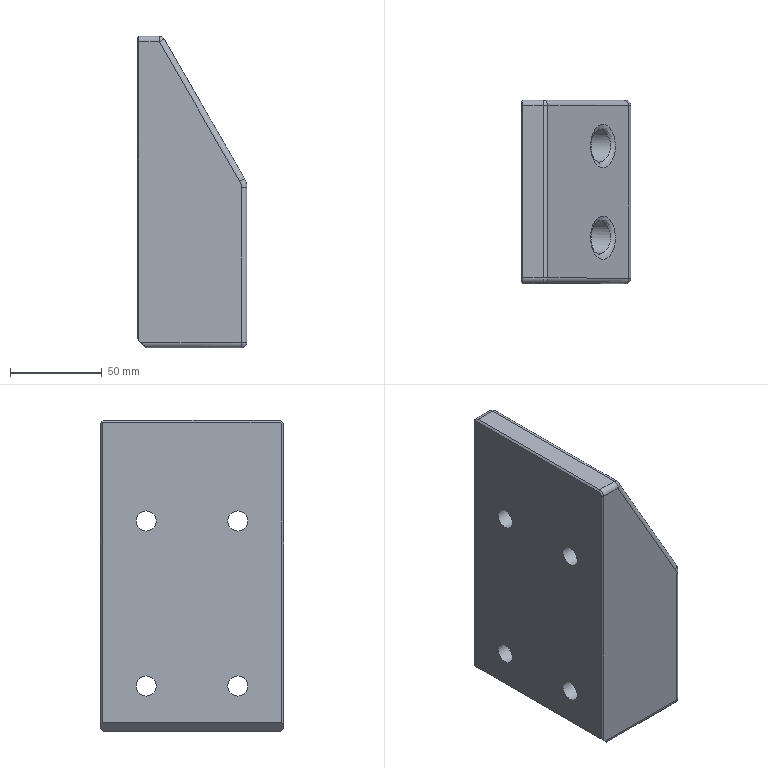Part | NX | features MAIN_BODY 2 | 1 solid | 45 faces | box 60 x 100 x 170 mm | volume 792826 mm3 | cylinder 19 | plane 15 | torus 4 | sphere 4 | spline 2 | cone 1 | commonest cylinder face diameters 6 x10 11 x4 17.5 x4 20 x1
STEP:
#1=CARTESIAN_POINT('',(997.,50.,-147.));
#2=VERTEX_POINT('',#1);
#3=CARTESIAN_POINT('',(996.,50.,-146.));
#4=VERTEX_POINT('',#3);
#5=CARTESIAN_POINT('',(995.,50.,-145.));
#6=DIRECTION('',(0.7071,0.,-0.7071));
#7=VECTOR('',#6,1000.);
#8=LINE('',#5,#7);
#9=EDGE_CURVE('',#2,#4,#8,.F.);
#10=ORIENTED_EDGE('',*,*,#9,.T.);
#11=CARTESIAN_POINT('',(996.,50.,17.));
#12=VERTEX_POINT('',#11);
#13=CARTESIAN_POINT('',(996.,50.,-335.));
#14=DIRECTION('',(0.,0.,1.));
#15=VECTOR('',#14,1000.);
#16=LINE('',#13,#15);
#17=EDGE_CURVE('',#4,#12,#16,.T.);
#18=ORIENTED_EDGE('',*,*,#17,.T.);
#19=CARTESIAN_POINT('',(1007.08,50.,17.));
#20=VERTEX_POINT('',#19);
#21=CARTESIAN_POINT('',(865.,50.,17.));
#22=DIRECTION('',(1.,0.,0.));
#23=VECTOR('',#22,1000.);
#24=LINE('',#21,#23);
#25=EDGE_CURVE('',#12,#20,#24,.T.);
#26=ORIENTED_EDGE('',*,*,#25,.T.);
#27=CARTESIAN_POINT('',(1051.062,50.,-59.179));
#28=VERTEX_POINT('',#27);
#29=CARTESIAN_POINT('',(1051.062,50.,-59.179));
#30=DIRECTION('',(0.5,0.,-0.866));
#31=VECTOR('',#30,1000.);
#32=LINE('',#29,#31);
#33=EDGE_CURVE('',#20,#28,#32,.T.);
#34=ORIENTED_EDGE('',*,*,#33,.T.);
#35=CARTESIAN_POINT('',(1052.,50.,-62.679));
#36=VERTEX_POINT('',#35);
#37=CARTESIAN_POINT('',(1045.,50.,-62.679));
#38=DIRECTION('',(0.,-1.,0.));
#39=DIRECTION('',(1.,0.,0.));
#40=AXIS2_PLACEMENT_3D('',#37,#38,#39);
#41=CIRCLE('',#40,7.);
#42=EDGE_CURVE('',#28,#36,#41,.F.);
#43=ORIENTED_EDGE('',*,*,#42,.T.);
#44=CARTESIAN_POINT('',(1052.,50.,-147.));
#45=VERTEX_POINT('',#44);
#46=CARTESIAN_POINT('',(1052.,50.,-335.));
#47=DIRECTION('',(0.,0.,-1.));
#48=VECTOR('',#47,1000.);
#49=LINE('',#46,#48);
#50=EDGE_CURVE('',#36,#45,#49,.T.);
#51=ORIENTED_EDGE('',*,*,#50,.T.);
#52=CARTESIAN_POINT('',(865.,50.,-147.));
#53=DIRECTION('',(-1.,0.,0.));
#54=VECTOR('',#53,1000.);
#55=LINE('',#52,#54);
#56=EDGE_CURVE('',#45,#2,#55,.T.);
#57=ORIENTED_EDGE('',*,*,#56,.T.);
#58=EDGE_LOOP('',(#10,#18,#26,#34,#43,#51,#57));
#59=FACE_BOUND('',#58,.T.);
#60=CARTESIAN_POINT('',(865.,50.,-335.));
#61=DIRECTION('',(0.,-1.,0.));
#62=DIRECTION('',(0.,0.,1.));
#63=AXIS2_PLACEMENT_3D('',#60,#61,#62);
#64=PLANE('',#63);
#65=ADVANCED_FACE('',(#59),#64,.F.);
#66=CARTESIAN_POINT('',(997.,-50.,-147.));
#67=VERTEX_POINT('',#66);
#68=CARTESIAN_POINT('',(996.,-50.,-146.));
#69=VERTEX_POINT('',#68);
#70=CARTESIAN_POINT('',(995.,-50.,-145.));
#71=DIRECTION('',(-0.7071,0.,0.7071));
#72=VECTOR('',#71,1000.);
#73=LINE('',#70,#72);
#74=EDGE_CURVE('',#67,#69,#73,.T.);
#75=ORIENTED_EDGE('',*,*,#74,.F.);
#76=CARTESIAN_POINT('',(1052.,-50.,-147.));
#77=VERTEX_POINT('',#76);
#78=CARTESIAN_POINT('',(865.,-50.,-147.));
#79=DIRECTION('',(-1.,0.,0.));
#80=VECTOR('',#79,1000.);
#81=LINE('',#78,#80);
#82=EDGE_CURVE('',#77,#67,#81,.T.);
#83=ORIENTED_EDGE('',*,*,#82,.F.);
#84=CARTESIAN_POINT('',(1052.,-50.,-62.679));
#85=VERTEX_POINT('',#84);
#86=CARTESIAN_POINT('',(1052.,-50.,-335.));
#87=DIRECTION('',(0.,0.,1.));
#88=VECTOR('',#87,1000.);
#89=LINE('',#86,#88);
#90=EDGE_CURVE('',#85,#77,#89,.F.);
#91=ORIENTED_EDGE('',*,*,#90,.F.);
#92=CARTESIAN_POINT('',(1051.062,-50.,-59.179));
#93=VERTEX_POINT('',#92);
#94=CARTESIAN_POINT('',(1045.,-50.,-62.679));
#95=DIRECTION('',(0.,1.,0.));
#96=DIRECTION('',(-1.,0.,0.));
#97=AXIS2_PLACEMENT_3D('',#94,#95,#96);
#98=CIRCLE('',#97,7.);
#99=EDGE_CURVE('',#93,#85,#98,.T.);
#100=ORIENTED_EDGE('',*,*,#99,.F.);
#101=CARTESIAN_POINT('',(1007.08,-50.,17.));
#102=VERTEX_POINT('',#101);
#103=CARTESIAN_POINT('',(1051.062,-50.,-59.179));
#104=DIRECTION('',(-0.5,0.,0.866));
#105=VECTOR('',#104,1000.);
#106=LINE('',#103,#105);
#107=EDGE_CURVE('',#102,#93,#106,.F.);
#108=ORIENTED_EDGE('',*,*,#107,.F.);
#109=CARTESIAN_POINT('',(996.,-50.,17.));
#110=VERTEX_POINT('',#109);
#111=CARTESIAN_POINT('',(865.,-50.,17.));
#112=DIRECTION('',(1.,0.,0.));
#113=VECTOR('',#112,1000.);
#114=LINE('',#111,#113);
#115=EDGE_CURVE('',#110,#102,#114,.T.);
#116=ORIENTED_EDGE('',*,*,#115,.F.);
#117=CARTESIAN_POINT('',(996.,-50.,-335.));
#118=DIRECTION('',(0.,0.,-1.));
#119=VECTOR('',#118,1000.);
#120=LINE('',#117,#119);
#121=EDGE_CURVE('',#69,#110,#120,.F.);
#122=ORIENTED_EDGE('',*,*,#121,.F.);
#123=EDGE_LOOP('',(#75,#83,#91,#100,#108,#116,#122));
#124=FACE_BOUND('',#123,.T.);
#125=CARTESIAN_POINT('',(865.,-50.,-335.));
#126=DIRECTION('',(0.,-1.,0.));
#127=DIRECTION('',(0.,0.,1.));
#128=AXIS2_PLACEMENT_3D('',#125,#126,#127);
#129=PLANE('',#128);
#130=ADVANCED_FACE('',(#124),#129,.T.);
#131=CARTESIAN_POINT('',(1055.,25.,-136.75));
#132=VERTEX_POINT('',#131);
#133=CARTESIAN_POINT('',(1055.,25.,-125.));
#134=DIRECTION('',(1.,0.,0.));
#135=DIRECTION('',(0.,0.,-1.));
#136=AXIS2_PLACEMENT_3D('',#133,#134,#135);
#137=CIRCLE('',#136,11.75);
#138=EDGE_CURVE('',#132,#132,#137,.T.);
#139=ORIENTED_EDGE('',*,*,#138,.F.);
#140=EDGE_LOOP('',(#139));
#141=FACE_BOUND('',#140,.T.);
#142=CARTESIAN_POINT('',(1055.,-25.,-136.75));
#143=VERTEX_POINT('',#142);
#144=CARTESIAN_POINT('',(1055.,-25.,-125.));
#145=DIRECTION('',(1.,0.,0.));
#146=DIRECTION('',(0.,0.,-1.));
#147=AXIS2_PLACEMENT_3D('',#144,#145,#146);
#148=CIRCLE('',#147,11.75);
#149=EDGE_CURVE('',#143,#143,#148,.T.);
#150=ORIENTED_EDGE('',*,*,#149,.F.);
#151=EDGE_LOOP('',(#150));
#152=FACE_BOUND('',#151,.T.);
#153=CARTESIAN_POINT('',(1055.,47.,-147.));
#154=VERTEX_POINT('',#153);
#155=CARTESIAN_POINT('',(1055.,-47.,-147.));
#156=VERTEX_POINT('',#155);
#157=CARTESIAN_POINT('',(1055.,0.,-147.));
#158=DIRECTION('',(0.,-1.,0.));
#159=VECTOR('',#158,1000.);
#160=LINE('',#157,#159);
#161=EDGE_CURVE('',#154,#156,#160,.T.);
#162=ORIENTED_EDGE('',*,*,#161,.F.);
#163=CARTESIAN_POINT('',(1055.,47.,-62.679));
#164=VERTEX_POINT('',#163);
#165=CARTESIAN_POINT('',(1055.,47.,-105.));
#166=DIRECTION('',(0.,0.,-1.));
#167=VECTOR('',#166,1000.);
#168=LINE('',#165,#167);
#169=EDGE_CURVE('',#154,#164,#168,.F.);
#170=ORIENTED_EDGE('',*,*,#169,.T.);
#171=CARTESIAN_POINT('',(1055.,-47.,-62.679));
#172=VERTEX_POINT('',#171);
#173=CARTESIAN_POINT('',(1055.,-40.,-62.679));
#174=DIRECTION('',(0.,1.,0.));
#175=VECTOR('',#174,1000.);
#176=LINE('',#173,#175);
#177=EDGE_CURVE('',#164,#172,#176,.F.);
#178=ORIENTED_EDGE('',*,*,#177,.T.);
#179=CARTESIAN_POINT('',(1055.,-47.,-105.));
#180=DIRECTION('',(0.,0.,-1.));
#181=VECTOR('',#180,1000.);
#182=LINE('',#179,#181);
#183=EDGE_CURVE('',#156,#172,#182,.F.);
#184=ORIENTED_EDGE('',*,*,#183,.F.);
#185=EDGE_LOOP('',(#162,#170,#178,#184));
#186=FACE_BOUND('',#185,.T.);
#187=CARTESIAN_POINT('',(1055.,0.,-105.));
#188=DIRECTION('',(-1.,0.,0.));
#189=DIRECTION('',(0.,1.,0.));
#190=AXIS2_PLACEMENT_3D('',#187,#188,#189);
#191=PLANE('',#190);
#192=ADVANCED_FACE('',(#141,#152,#186),#191,.F.);
#193=CARTESIAN_POINT('',(1043.886,25.,-43.75));
#194=VERTEX_POINT('',#193);
#195=CARTESIAN_POINT('',(1037.102,25.,-35.));
#196=DIRECTION('',(0.7903,0.,0.6127));
#197=DIRECTION('',(0.6127,0.,-0.7903));
#198=AXIS2_PLACEMENT_3D('',#195,#196,#197);
#199=ELLIPSE('',#198,11.072,8.75);
#200=EDGE_CURVE('',#194,#194,#199,.F.);
#201=ORIENTED_EDGE('',*,*,#200,.F.);
#202=EDGE_LOOP('',(#201));
#203=FACE_BOUND('',#202,.T.);
#204=CARTESIAN_POINT('',(1015.,25.,-26.25));
#205=VERTEX_POINT('',#204);
#206=CARTESIAN_POINT('',(1015.,25.,-35.));
#207=DIRECTION('',(1.,0.,0.));
#208=DIRECTION('',(0.,0.,1.));
#209=AXIS2_PLACEMENT_3D('',#206,#207,#208);
#210=CIRCLE('',#209,8.75);
#211=EDGE_CURVE('',#205,#205,#210,.T.);
#212=ORIENTED_EDGE('',*,*,#211,.F.);
#213=EDGE_LOOP('',(#212));
#214=FACE_BOUND('',#213,.T.);
#215=CARTESIAN_POINT('',(1020.,25.,-35.));
#216=DIRECTION('',(1.,0.,0.));
#217=DIRECTION('',(0.,0.,1.));
#218=AXIS2_PLACEMENT_3D('',#215,#216,#217);
#219=CYLINDRICAL_SURFACE('',#218,8.75);
#220=ADVANCED_FACE('',(#203,#214),#219,.F.);
#221=CARTESIAN_POINT('',(1043.886,-25.,-43.75));
#222=VERTEX_POINT('',#221);
#223=CARTESIAN_POINT('',(1037.102,-25.,-35.));
#224=DIRECTION('',(0.7903,0.,0.6127));
#225=DIRECTION('',(0.6127,0.,-0.7903));
#226=AXIS2_PLACEMENT_3D('',#223,#224,#225);
#227=ELLIPSE('',#226,11.072,8.75);
#228=EDGE_CURVE('',#222,#222,#227,.F.);
#229=ORIENTED_EDGE('',*,*,#228,.F.);
#230=EDGE_LOOP('',(#229));
#231=FACE_BOUND('',#230,.T.);
#232=CARTESIAN_POINT('',(1015.,-25.,-26.25));
#233=VERTEX_POINT('',#232);
#234=CARTESIAN_POINT('',(1015.,-25.,-35.));
#235=DIRECTION('',(1.,0.,0.));
#236=DIRECTION('',(0.,0.,1.));
#237=AXIS2_PLACEMENT_3D('',#234,#235,#236);
#238=CIRCLE('',#237,8.75);
#239=EDGE_CURVE('',#233,#233,#238,.T.);
#240=ORIENTED_EDGE('',*,*,#239,.F.);
#241=EDGE_LOOP('',(#240));
#242=FACE_BOUND('',#241,.T.);
#243=CARTESIAN_POINT('',(1020.,-25.,-35.));
#244=DIRECTION('',(1.,0.,0.));
#245=DIRECTION('',(0.,0.,1.));
#246=AXIS2_PLACEMENT_3D('',#243,#244,#245);
#247=CYLINDRICAL_SURFACE('',#246,8.75);
#248=ADVANCED_FACE('',(#231,#242),#247,.F.);
#249=CARTESIAN_POINT('',(995.,25.,-29.5));
#250=VERTEX_POINT('',#249);
#251=CARTESIAN_POINT('',(995.,25.,-35.));
#252=DIRECTION('',(1.,0.,0.));
#253=DIRECTION('',(0.,0.,1.));
#254=AXIS2_PLACEMENT_3D('',#251,#252,#253);
#255=CIRCLE('',#254,5.5);
#256=EDGE_CURVE('',#250,#250,#255,.F.);
#257=ORIENTED_EDGE('',*,*,#256,.F.);
#258=EDGE_LOOP('',(#257));
#259=FACE_BOUND('',#258,.T.);
#260=CARTESIAN_POINT('',(995.,25.,-119.5));
#261=VERTEX_POINT('',#260);
#262=CARTESIAN_POINT('',(995.,25.,-125.));
#263=DIRECTION('',(1.,0.,0.));
#264=DIRECTION('',(0.,0.,1.));
#265=AXIS2_PLACEMENT_3D('',#262,#263,#264);
#266=CIRCLE('',#265,5.5);
#267=EDGE_CURVE('',#261,#261,#266,.F.);
#268=ORIENTED_EDGE('',*,*,#267,.F.);
#269=EDGE_LOOP('',(#268));
#270=FACE_BOUND('',#269,.T.);
#271=CARTESIAN_POINT('',(995.,-25.,-119.5));
#272=VERTEX_POINT('',#271);
#273=CARTESIAN_POINT('',(995.,-25.,-125.));
#274=DIRECTION('',(1.,0.,0.));
#275=DIRECTION('',(0.,0.,1.));
#276=AXIS2_PLACEMENT_3D('',#273,#274,#275);
#277=CIRCLE('',#276,5.5);
#278=EDGE_CURVE('',#272,#272,#277,.F.);
#279=ORIENTED_EDGE('',*,*,#278,.F.);
#280=EDGE_LOOP('',(#279));
#281=FACE_BOUND('',#280,.T.);
#282=CARTESIAN_POINT('',(995.,49.,19.));
#283=VERTEX_POINT('',#282);
#284=CARTESIAN_POINT('',(995.,-47.,19.));
#285=VERTEX_POINT('',#284);
#286=CARTESIAN_POINT('',(995.,95.,19.));
#287=DIRECTION('',(0.,-1.,0.));
#288=VECTOR('',#287,1000.);
#289=LINE('',#286,#288);
#290=EDGE_CURVE('',#283,#285,#289,.T.);
#291=ORIENTED_EDGE('',*,*,#290,.F.);
#292=CARTESIAN_POINT('',(995.,49.,-145.));
#293=VERTEX_POINT('',#292);
#294=CARTESIAN_POINT('',(995.,49.,-335.));
#295=DIRECTION('',(0.,0.,-1.));
#296=VECTOR('',#295,1000.);
#297=LINE('',#294,#296);
#298=EDGE_CURVE('',#283,#293,#297,.T.);
#299=ORIENTED_EDGE('',*,*,#298,.T.);
#300=CARTESIAN_POINT('',(995.,-49.,-145.));
#301=VERTEX_POINT('',#300);
#302=CARTESIAN_POINT('',(995.,95.,-145.));
#303=DIRECTION('',(0.,1.,0.));
#304=VECTOR('',#303,1000.);
#305=LINE('',#302,#304);
#306=EDGE_CURVE('',#301,#293,#305,.T.);
#307=ORIENTED_EDGE('',*,*,#306,.F.);
#308=CARTESIAN_POINT('',(995.,-49.,17.));
#309=VERTEX_POINT('',#308);
#310=CARTESIAN_POINT('',(995.,-49.,-335.));
#311=DIRECTION('',(0.,0.,-1.));
#312=VECTOR('',#311,1000.);
#313=LINE('',#310,#312);
#314=EDGE_CURVE('',#309,#301,#313,.T.);
#315=ORIENTED_EDGE('',*,*,#314,.F.);
#316=CARTESIAN_POINT('',(995.,-47.,17.));
#317=DIRECTION('',(-1.,0.,0.));
#318=DIRECTION('',(0.,0.,1.));
#319=AXIS2_PLACEMENT_3D('',#316,#317,#318);
#320=CIRCLE('',#319,2.);
#321=EDGE_CURVE('',#285,#309,#320,.F.);
#322=ORIENTED_EDGE('',*,*,#321,.F.);
#323=EDGE_LOOP('',(#291,#299,#307,#315,#322));
#324=FACE_BOUND('',#323,.T.);
#325=CARTESIAN_POINT('',(995.,-25.,-29.5));
#326=VERTEX_POINT('',#325);
#327=CARTESIAN_POINT('',(995.,-25.,-35.));
#328=DIRECTION('',(1.,0.,0.));
#329=DIRECTION('',(0.,0.,1.));
#330=AXIS2_PLACEMENT_3D('',#327,#328,#329);
#331=CIRCLE('',#330,5.5);
#332=EDGE_CURVE('',#326,#326,#331,.F.);
#333=ORIENTED_EDGE('',*,*,#332,.F.);
#334=EDGE_LOOP('',(#333));
#335=FACE_BOUND('',#334,.T.);
#336=CARTESIAN_POINT('',(995.,95.,-335.));
#337=DIRECTION('',(1.,0.,0.));
#338=DIRECTION('',(0.,-1.,0.));
#339=AXIS2_PLACEMENT_3D('',#336,#337,#338);
#340=PLANE('',#339);
#341=ADVANCED_FACE('',(#259,#270,#281,#324,#335),#340,.F.);
#342=CARTESIAN_POINT('',(1007.08,47.,20.));
#343=VERTEX_POINT('',#342);
#344=CARTESIAN_POINT('',(1007.08,-47.,20.));
#345=VERTEX_POINT('',#344);
#346=CARTESIAN_POINT('',(1007.08,-47.,20.));
#347=DIRECTION('',(0.,-1.,0.));
#348=VECTOR('',#347,1000.);
#349=LINE('',#346,#348);
#350=EDGE_CURVE('',#343,#345,#349,.T.);
#351=ORIENTED_EDGE('',*,*,#350,.F.);
#352=CARTESIAN_POINT('',(996.,47.,20.));
#353=VERTEX_POINT('',#352);
#354=CARTESIAN_POINT('',(850.,47.,20.));
#355=DIRECTION('',(1.,0.,0.));
#356=VECTOR('',#355,1000.);
#357=LINE('',#354,#356);
#358=EDGE_CURVE('',#343,#353,#357,.F.);
#359=ORIENTED_EDGE('',*,*,#358,.T.);
#360=CARTESIAN_POINT('',(996.,-47.,20.));
#361=VERTEX_POINT('',#360);
#362=CARTESIAN_POINT('',(996.,-5.,20.));
#363=DIRECTION('',(0.,1.,0.));
#364=VECTOR('',#363,1000.);
#365=LINE('',#362,#364);
#366=EDGE_CURVE('',#361,#353,#365,.T.);
#367=ORIENTED_EDGE('',*,*,#366,.F.);
#368=CARTESIAN_POINT('',(850.,-47.,20.));
#369=DIRECTION('',(-1.,0.,0.));
#370=VECTOR('',#369,1000.);
#371=LINE('',#368,#370);
#372=EDGE_CURVE('',#345,#361,#371,.T.);
#373=ORIENTED_EDGE('',*,*,#372,.F.);
#374=EDGE_LOOP('',(#351,#359,#367,#373));
#375=FACE_BOUND('',#374,.T.);
#376=CARTESIAN_POINT('',(850.,-5.,20.));
#377=DIRECTION('',(0.,0.,-1.));
#378=DIRECTION('',(0.4226,-0.9063,0.));
#379=AXIS2_PLACEMENT_3D('',#376,#377,#378);
#380=PLANE('',#379);
#381=ADVANCED_FACE('',(#375),#380,.F.);
#382=CARTESIAN_POINT('',(1000.,47.,-150.));
#383=VERTEX_POINT('',#382);
#384=CARTESIAN_POINT('',(1000.,-47.,-150.));
#385=VERTEX_POINT('',#384);
#386=CARTESIAN_POINT('',(1000.,75.625,-150.));
#387=DIRECTION('',(0.,-1.,0.));
#388=VECTOR('',#387,1000.);
#389=LINE('',#386,#388);
#390=EDGE_CURVE('',#383,#385,#389,.T.);
#391=ORIENTED_EDGE('',*,*,#390,.F.);
#392=CARTESIAN_POINT('',(1052.,47.,-150.));
#393=VERTEX_POINT('',#392);
#394=CARTESIAN_POINT('',(906.301,47.,-150.));
#395=DIRECTION('',(-1.,0.,0.));
#396=VECTOR('',#395,1000.);
#397=LINE('',#394,#396);
#398=EDGE_CURVE('',#383,#393,#397,.F.);
#399=ORIENTED_EDGE('',*,*,#398,.T.);
#400=CARTESIAN_POINT('',(1052.,-47.,-150.));
#401=VERTEX_POINT('',#400);
#402=CARTESIAN_POINT('',(1052.,75.625,-150.));
#403=DIRECTION('',(0.,-1.,0.));
#404=VECTOR('',#403,1000.);
#405=LINE('',#402,#404);
#406=EDGE_CURVE('',#401,#393,#405,.F.);
#407=ORIENTED_EDGE('',*,*,#406,.F.);
#408=CARTESIAN_POINT('',(906.301,-47.,-150.));
#409=DIRECTION('',(1.,0.,0.));
#410=VECTOR('',#409,1000.);
#411=LINE('',#408,#410);
#412=EDGE_CURVE('',#385,#401,#411,.T.);
#413=ORIENTED_EDGE('',*,*,#412,.F.);
#414=EDGE_LOOP('',(#391,#399,#407,#413));
#415=FACE_BOUND('',#414,.T.);
#416=CARTESIAN_POINT('',(906.301,75.625,-150.));
#417=DIRECTION('',(0.,0.,1.));
#418=DIRECTION('',(0.866,0.5,0.));
#419=AXIS2_PLACEMENT_3D('',#416,#417,#418);
#420=PLANE('',#419);
#421=ADVANCED_FACE('',(#415),#420,.F.);
#422=CARTESIAN_POINT('',(1015.,-25.,-119.5));
#423=VERTEX_POINT('',#422);
#424=CARTESIAN_POINT('',(1015.,-25.,-125.));
#425=DIRECTION('',(-1.,0.,0.));
#426=DIRECTION('',(0.,0.,1.));
#427=AXIS2_PLACEMENT_3D('',#424,#425,#426);
#428=CIRCLE('',#427,5.5);
#429=EDGE_CURVE('',#423,#423,#428,.F.);
#430=ORIENTED_EDGE('',*,*,#429,.T.);
#431=EDGE_LOOP('',(#430));
#432=FACE_BOUND('',#431,.T.);
#433=ORIENTED_EDGE('',*,*,#278,.T.);
#434=EDGE_LOOP('',(#433));
#435=FACE_BOUND('',#434,.T.);
#436=CARTESIAN_POINT('',(870.,-25.,-125.));
#437=DIRECTION('',(-1.,0.,0.));
#438=DIRECTION('',(0.,-1.,0.));
#439=AXIS2_PLACEMENT_3D('',#436,#437,#438);
#440=CYLINDRICAL_SURFACE('',#439,5.5);
#441=ADVANCED_FACE('',(#432,#435),#440,.F.);
#442=ORIENTED_EDGE('',*,*,#429,.F.);
#443=EDGE_LOOP('',(#442));
#444=FACE_BOUND('',#443,.T.);
#445=CARTESIAN_POINT('',(1015.,-25.,-116.25));
#446=VERTEX_POINT('',#445);
#447=CARTESIAN_POINT('',(1015.,-25.,-125.));
#448=DIRECTION('',(-1.,0.,0.));
#449=DIRECTION('',(0.,0.,1.));
#450=AXIS2_PLACEMENT_3D('',#447,#448,#449);
#451=CIRCLE('',#450,8.75);
#452=EDGE_CURVE('',#446,#446,#451,.F.);
#453=ORIENTED_EDGE('',*,*,#452,.T.);
#454=EDGE_LOOP('',(#453));
#455=FACE_BOUND('',#454,.T.);
#456=CARTESIAN_POINT('',(1015.,-5.,-75.));
#457=DIRECTION('',(-1.,0.,0.));
#458=DIRECTION('',(0.,-1.,0.));
#459=AXIS2_PLACEMENT_3D('',#456,#457,#458);
#460=PLANE('',#459);
#461=ADVANCED_FACE('',(#444,#455),#460,.F.);
#462=CARTESIAN_POINT('',(1052.,-25.,-133.75));
#463=VERTEX_POINT('',#462);
#464=CARTESIAN_POINT('',(1052.,-25.,-125.));
#465=DIRECTION('',(1.,0.,0.));
#466=DIRECTION('',(0.,0.,-1.));
#467=AXIS2_PLACEMENT_3D('',#464,#465,#466);
#468=CIRCLE('',#467,8.75);
#469=EDGE_CURVE('',#463,#463,#468,.F.);
#470=ORIENTED_EDGE('',*,*,#469,.F.);
#471=EDGE_LOOP('',(#470));
#472=FACE_BOUND('',#471,.T.);
#473=ORIENTED_EDGE('',*,*,#452,.F.);
#474=EDGE_LOOP('',(#473));
#475=FACE_BOUND('',#474,.T.);
#476=CARTESIAN_POINT('',(1075.,-25.,-125.));
#477=DIRECTION('',(-1.,0.,0.));
#478=DIRECTION('',(0.,-1.,0.));
#479=AXIS2_PLACEMENT_3D('',#476,#477,#478);
#480=CYLINDRICAL_SURFACE('',#479,8.75);
#481=ADVANCED_FACE('',(#472,#475),#480,.F.);
#482=CARTESIAN_POINT('',(1015.,25.,-119.5));
#483=VERTEX_POINT('',#482);
#484=CARTESIAN_POINT('',(1015.,25.,-125.));
#485=DIRECTION('',(-1.,0.,0.));
#486=DIRECTION('',(0.,0.,1.));
#487=AXIS2_PLACEMENT_3D('',#484,#485,#486);
#488=CIRCLE('',#487,5.5);
#489=EDGE_CURVE('',#483,#483,#488,.F.);
#490=ORIENTED_EDGE('',*,*,#489,.T.);
#491=EDGE_LOOP('',(#490));
#492=FACE_BOUND('',#491,.T.);
#493=ORIENTED_EDGE('',*,*,#267,.T.);
#494=EDGE_LOOP('',(#493));
#495=FACE_BOUND('',#494,.T.);
#496=CARTESIAN_POINT('',(870.,25.,-125.));
#497=DIRECTION('',(-1.,0.,0.));
#498=DIRECTION('',(0.,-1.,0.));
#499=AXIS2_PLACEMENT_3D('',#496,#497,#498);
#500=CYLINDRICAL_SURFACE('',#499,5.5);
#501=ADVANCED_FACE('',(#492,#495),#500,.F.);
#502=ORIENTED_EDGE('',*,*,#489,.F.);
#503=EDGE_LOOP('',(#502));
#504=FACE_BOUND('',#503,.T.);
#505=CARTESIAN_POINT('',(1015.,25.,-116.25));
#506=VERTEX_POINT('',#505);
#507=CARTESIAN_POINT('',(1015.,25.,-125.));
#508=DIRECTION('',(-1.,0.,0.));
#509=DIRECTION('',(0.,0.,1.));
#510=AXIS2_PLACEMENT_3D('',#507,#508,#509);
#511=CIRCLE('',#510,8.75);
#512=EDGE_CURVE('',#506,#506,#511,.F.);
#513=ORIENTED_EDGE('',*,*,#512,.T.);
#514=EDGE_LOOP('',(#513));
#515=FACE_BOUND('',#514,.T.);
#516=CARTESIAN_POINT('',(1015.,80.,-75.));
#517=DIRECTION('',(-1.,0.,0.));
#518=DIRECTION('',(0.,-1.,0.));
#519=AXIS2_PLACEMENT_3D('',#516,#517,#518);
#520=PLANE('',#519);
#521=ADVANCED_FACE('',(#504,#515),#520,.F.);
#522=CARTESIAN_POINT('',(1052.,25.,-133.75));
#523=VERTEX_POINT('',#522);
#524=CARTESIAN_POINT('',(1052.,25.,-125.));
#525=DIRECTION('',(1.,0.,0.));
#526=DIRECTION('',(0.,0.,-1.));
#527=AXIS2_PLACEMENT_3D('',#524,#525,#526);
#528=CIRCLE('',#527,8.75);
#529=EDGE_CURVE('',#523,#523,#528,.F.);
#530=ORIENTED_EDGE('',*,*,#529,.F.);
#531=EDGE_LOOP('',(#530));
#532=FACE_BOUND('',#531,.T.);
#533=ORIENTED_EDGE('',*,*,#512,.F.);
#534=EDGE_LOOP('',(#533));
#535=FACE_BOUND('',#534,.T.);
#536=CARTESIAN_POINT('',(1075.,25.,-125.));
#537=DIRECTION('',(-1.,0.,0.));
#538=DIRECTION('',(0.,-1.,0.));
#539=AXIS2_PLACEMENT_3D('',#536,#537,#538);
#540=CYLINDRICAL_SURFACE('',#539,8.75);
#541=ADVANCED_FACE('',(#532,#535),#540,.F.);
#542=ORIENTED_EDGE('',*,*,#256,.T.);
#543=EDGE_LOOP('',(#542));
#544=FACE_BOUND('',#543,.T.);
#545=CARTESIAN_POINT('',(1015.,25.,-29.5));
#546=VERTEX_POINT('',#545);
#547=CARTESIAN_POINT('',(1015.,25.,-35.));
#548=DIRECTION('',(1.,0.,0.));
#549=DIRECTION('',(0.,0.,1.));
#550=AXIS2_PLACEMENT_3D('',#547,#548,#549);
#551=CIRCLE('',#550,5.5);
#552=EDGE_CURVE('',#546,#546,#551,.T.);
#553=ORIENTED_EDGE('',*,*,#552,.T.);
#554=EDGE_LOOP('',(#553));
#555=FACE_BOUND('',#554,.T.);
#556=CARTESIAN_POINT('',(990.,25.,-35.));
#557=DIRECTION('',(1.,0.,0.));
#558=DIRECTION('',(0.,0.,1.));
#559=AXIS2_PLACEMENT_3D('',#556,#557,#558);
#560=CYLINDRICAL_SURFACE('',#559,5.5);
#561=ADVANCED_FACE('',(#544,#555),#560,.F.);
#562=ORIENTED_EDGE('',*,*,#211,.T.);
#563=EDGE_LOOP('',(#562));
#564=FACE_BOUND('',#563,.T.);
#565=ORIENTED_EDGE('',*,*,#552,.F.);
#566=EDGE_LOOP('',(#565));
#567=FACE_BOUND('',#566,.T.);
#568=CARTESIAN_POINT('',(1015.,50.,-50.));
#569=DIRECTION('',(1.,0.,0.));
#570=DIRECTION('',(0.,0.,1.));
#571=AXIS2_PLACEMENT_3D('',#568,#569,#570);
#572=PLANE('',#571);
#573=ADVANCED_FACE('',(#564,#567),#572,.T.);
#574=ORIENTED_EDGE('',*,*,#332,.T.);
#575=EDGE_LOOP('',(#574));
#576=FACE_BOUND('',#575,.T.);
#577=CARTESIAN_POINT('',(1015.,-25.,-29.5));
#578=VERTEX_POINT('',#577);
#579=CARTESIAN_POINT('',(1015.,-25.,-35.));
#580=DIRECTION('',(1.,0.,0.));
#581=DIRECTION('',(0.,0.,1.));
#582=AXIS2_PLACEMENT_3D('',#579,#580,#581);
#583=CIRCLE('',#582,5.5);
#584=EDGE_CURVE('',#578,#578,#583,.T.);
#585=ORIENTED_EDGE('',*,*,#584,.T.);
#586=EDGE_LOOP('',(#585));
#587=FACE_BOUND('',#586,.T.);
#588=CARTESIAN_POINT('',(990.,-25.,-35.));
#589=DIRECTION('',(1.,0.,0.));
#590=DIRECTION('',(0.,0.,1.));
#591=AXIS2_PLACEMENT_3D('',#588,#589,#590);
#592=CYLINDRICAL_SURFACE('',#591,5.5);
#593=ADVANCED_FACE('',(#576,#587),#592,.F.);
#594=ORIENTED_EDGE('',*,*,#239,.T.);
#595=EDGE_LOOP('',(#594));
#596=FACE_BOUND('',#595,.T.);
#597=ORIENTED_EDGE('',*,*,#584,.F.);
#598=EDGE_LOOP('',(#597));
#599=FACE_BOUND('',#598,.T.);
#600=CARTESIAN_POINT('',(1015.,-5.,-50.));
#601=DIRECTION('',(1.,0.,0.));
#602=DIRECTION('',(0.,0.,1.));
#603=AXIS2_PLACEMENT_3D('',#600,#601,#602);
#604=PLANE('',#603);
#605=ADVANCED_FACE('',(#596,#599),#604,.T.);
#606=CARTESIAN_POINT('',(1046.484,-25.,-45.25));
#607=VERTEX_POINT('',#606);
#608=CARTESIAN_POINT('',(1039.7,-25.,-33.5));
#609=DIRECTION('',(-0.866,0.,-0.5));
#610=DIRECTION('',(0.5,0.,-0.866));
#611=AXIS2_PLACEMENT_3D('',#608,#609,#610);
#612=ELLIPSE('',#611,13.568,11.75);
#613=EDGE_CURVE('',#607,#607,#612,.F.);
#614=ORIENTED_EDGE('',*,*,#613,.F.);
#615=EDGE_LOOP('',(#614));
#616=FACE_BOUND('',#615,.T.);
#617=CARTESIAN_POINT('',(1046.484,25.,-45.25));
#618=VERTEX_POINT('',#617);
#619=CARTESIAN_POINT('',(1039.7,25.,-33.5));
#620=DIRECTION('',(-0.866,0.,-0.5));
#621=DIRECTION('',(0.5,0.,-0.866));
#622=AXIS2_PLACEMENT_3D('',#619,#620,#621);
#623=ELLIPSE('',#622,13.568,11.75);
#624=EDGE_CURVE('',#618,#618,#623,.F.);
#625=ORIENTED_EDGE('',*,*,#624,.F.);
#626=EDGE_LOOP('',(#625));
#627=FACE_BOUND('',#626,.T.);
#628=CARTESIAN_POINT('',(1053.66,-47.,-57.679));
#629=VERTEX_POINT('',#628);
#630=CARTESIAN_POINT('',(1053.66,47.,-57.679));
#631=VERTEX_POINT('',#630);
#632=CARTESIAN_POINT('',(1053.66,60.,-57.679));
#633=DIRECTION('',(0.,1.,0.));
#634=VECTOR('',#633,1000.);
#635=LINE('',#632,#634);
#636=EDGE_CURVE('',#629,#631,#635,.T.);
#637=ORIENTED_EDGE('',*,*,#636,.T.);
#638=CARTESIAN_POINT('',(1009.678,47.,18.5));
#639=VERTEX_POINT('',#638);
#640=CARTESIAN_POINT('',(1009.678,47.,18.5));
#641=DIRECTION('',(0.5,0.,-0.866));
#642=VECTOR('',#641,1000.);
#643=LINE('',#640,#642);
#644=EDGE_CURVE('',#631,#639,#643,.F.);
#645=ORIENTED_EDGE('',*,*,#644,.T.);
#646=CARTESIAN_POINT('',(1009.678,-47.,18.5));
#647=VERTEX_POINT('',#646);
#648=CARTESIAN_POINT('',(1009.678,67.,18.5));
#649=DIRECTION('',(0.,-1.,0.));
#650=VECTOR('',#649,1000.);
#651=LINE('',#648,#650);
#652=EDGE_CURVE('',#647,#639,#651,.F.);
#653=ORIENTED_EDGE('',*,*,#652,.F.);
#654=CARTESIAN_POINT('',(1008.812,-47.,20.));
#655=DIRECTION('',(0.5,0.,-0.866));
#656=VECTOR('',#655,1000.);
#657=LINE('',#654,#656);
#658=EDGE_CURVE('',#629,#647,#657,.F.);
#659=ORIENTED_EDGE('',*,*,#658,.F.);
#660=EDGE_LOOP('',(#637,#645,#653,#659));
#661=FACE_BOUND('',#660,.T.);
#662=CARTESIAN_POINT('',(1094.748,-40.,-128.846));
#663=DIRECTION('',(0.866,0.,0.5));
#664=DIRECTION('',(0.5,0.,-0.866));
#665=AXIS2_PLACEMENT_3D('',#662,#663,#664);
#666=PLANE('',#665);
#667=ADVANCED_FACE('',(#616,#627,#661),#666,.T.);
#668=ORIENTED_EDGE('',*,*,#177,.F.);
#669=CARTESIAN_POINT('',(1045.,47.,-62.679));
#670=DIRECTION('',(0.,-1.,0.));
#671=DIRECTION('',(1.,0.,0.));
#672=AXIS2_PLACEMENT_3D('',#669,#670,#671);
#673=CIRCLE('',#672,10.);
#674=EDGE_CURVE('',#164,#631,#673,.T.);
#675=ORIENTED_EDGE('',*,*,#674,.T.);
#676=ORIENTED_EDGE('',*,*,#636,.F.);
#677=CARTESIAN_POINT('',(1045.,-47.,-62.679));
#678=DIRECTION('',(0.,1.,0.));
#679=DIRECTION('',(-1.,0.,0.));
#680=AXIS2_PLACEMENT_3D('',#677,#678,#679);
#681=CIRCLE('',#680,10.);
#682=EDGE_CURVE('',#172,#629,#681,.F.);
#683=ORIENTED_EDGE('',*,*,#682,.F.);
#684=EDGE_LOOP('',(#668,#675,#676,#683));
#685=FACE_BOUND('',#684,.T.);
#686=CARTESIAN_POINT('',(1045.,-40.,-62.679));
#687=DIRECTION('',(0.,-1.,0.));
#688=DIRECTION('',(1.,0.,0.));
#689=AXIS2_PLACEMENT_3D('',#686,#687,#688);
#690=CYLINDRICAL_SURFACE('',#689,10.);
#691=ADVANCED_FACE('',(#685),#690,.T.);
#692=ORIENTED_EDGE('',*,*,#306,.T.);
#693=CARTESIAN_POINT('',(1010.333,64.333,-160.333));
#694=DIRECTION('',(0.5774,0.5774,-0.5774));
#695=VECTOR('',#694,1000.);
#696=LINE('',#693,#695);
#697=EDGE_CURVE('',#293,#4,#696,.T.);
#698=ORIENTED_EDGE('',*,*,#697,.T.);
#699=ORIENTED_EDGE('',*,*,#9,.F.);
#700=CARTESIAN_POINT('',(997.,47.,-147.));
#701=DIRECTION('',(0.7071,0.,0.7071));
#702=DIRECTION('',(-0.7071,0.,0.7071));
#703=AXIS2_PLACEMENT_3D('',#700,#701,#702);
#704=ELLIPSE('',#703,4.243,3.);
#705=EDGE_CURVE('',#2,#383,#704,.F.);
#706=ORIENTED_EDGE('',*,*,#705,.T.);
#707=ORIENTED_EDGE('',*,*,#390,.T.);
#708=CARTESIAN_POINT('',(997.,-47.,-147.));
#709=DIRECTION('',(-0.7071,0.,-0.7071));
#710=DIRECTION('',(0.7071,0.,-0.7071));
#711=AXIS2_PLACEMENT_3D('',#708,#709,#710);
#712=ELLIPSE('',#711,4.243,3.);
#713=EDGE_CURVE('',#67,#385,#712,.F.);
#714=ORIENTED_EDGE('',*,*,#713,.F.);
#715=ORIENTED_EDGE('',*,*,#74,.T.);
#716=CARTESIAN_POINT('',(947.,-1.,-97.));
#717=DIRECTION('',(-0.5774,0.5774,0.5774));
#718=VECTOR('',#717,1000.);
#719=LINE('',#716,#718);
#720=EDGE_CURVE('',#301,#69,#719,.F.);
#721=ORIENTED_EDGE('',*,*,#720,.F.);
#722=EDGE_LOOP('',(#692,#698,#699,#706,#707,#714,#715,#721));
#723=FACE_BOUND('',#722,.T.);
#724=CARTESIAN_POINT('',(995.,95.,-145.));
#725=DIRECTION('',(0.7071,0.,0.7071));
#726=DIRECTION('',(-0.7071,0.,0.7071));
#727=AXIS2_PLACEMENT_3D('',#724,#725,#726);
#728=PLANE('',#727);
#729=ADVANCED_FACE('',(#723),#728,.F.);
#730=ORIENTED_EDGE('',*,*,#529,.T.);
#731=EDGE_LOOP('',(#730));
#732=FACE_BOUND('',#731,.T.);
#733=ORIENTED_EDGE('',*,*,#138,.T.);
#734=EDGE_LOOP('',(#733));
#735=FACE_BOUND('',#734,.T.);
#736=CARTESIAN_POINT('',(1052.,25.,-125.));
#737=DIRECTION('',(-1.,0.,0.));
#738=DIRECTION('',(0.,0.,-1.));
#739=AXIS2_PLACEMENT_3D('',#736,#737,#738);
#740=TOROIDAL_SURFACE('',#739,11.75,3.);
#741=ADVANCED_FACE('',(#732,#735),#740,.T.);
#742=ORIENTED_EDGE('',*,*,#469,.T.);
#743=EDGE_LOOP('',(#742));
#744=FACE_BOUND('',#743,.T.);
#745=ORIENTED_EDGE('',*,*,#149,.T.);
#746=EDGE_LOOP('',(#745));
#747=FACE_BOUND('',#746,.T.);
#748=CARTESIAN_POINT('',(1052.,-25.,-125.));
#749=DIRECTION('',(-1.,0.,0.));
#750=DIRECTION('',(0.,0.,-1.));
#751=AXIS2_PLACEMENT_3D('',#748,#749,#750);
#752=TOROIDAL_SURFACE('',#751,11.75,3.);
#753=ADVANCED_FACE('',(#744,#747),#752,.T.);
#754=ORIENTED_EDGE('',*,*,#613,.T.);
#755=EDGE_LOOP('',(#754));
#756=FACE_BOUND('',#755,.T.);
#757=ORIENTED_EDGE('',*,*,#228,.T.);
#758=EDGE_LOOP('',(#757));
#759=FACE_BOUND('',#758,.T.);
#760=CARTESIAN_POINT('',(1043.886,-25.,-43.75));
#761=CARTESIAN_POINT('',(1045.618,-25.,-43.75));
#762=CARTESIAN_POINT('',(1046.484,-25.,-45.25));
#763=CARTESIAN_POINT('',(1043.886,-27.287,-43.75));
#764=CARTESIAN_POINT('',(1045.618,-27.529,-43.75));
#765=CARTESIAN_POINT('',(1046.484,-28.07,-45.25));
#766=CARTESIAN_POINT('',(1042.417,-31.86,-41.855));
#767=CARTESIAN_POINT('',(1044.132,-32.862,-41.177));
#768=CARTESIAN_POINT('',(1045.015,-34.211,-42.705));
#769=CARTESIAN_POINT('',(1037.992,-34.214,-36.147));
#770=CARTESIAN_POINT('',(1040.176,-34.448,-34.323));
#771=CARTESIAN_POINT('',(1040.59,-37.373,-35.041));
#772=CARTESIAN_POINT('',(1034.438,-33.293,-31.564));
#773=CARTESIAN_POINT('',(1037.547,-32.534,-29.771));
#774=CARTESIAN_POINT('',(1037.036,-36.136,-28.886));
#775=CARTESIAN_POINT('',(1032.18,-31.349,-28.652));
#776=CARTESIAN_POINT('',(1036.152,-29.961,-27.354));
#777=CARTESIAN_POINT('',(1034.778,-33.525,-24.975));
#778=CARTESIAN_POINT('',(1030.671,-28.436,-26.706));
#779=CARTESIAN_POINT('',(1035.572,-27.215,-26.349));
#780=CARTESIAN_POINT('',(1033.27,-29.613,-22.362));
#781=CARTESIAN_POINT('',(1030.142,-25.,-26.022));
#782=CARTESIAN_POINT('',(1035.485,-25.,-26.198));
#783=CARTESIAN_POINT('',(1032.74,-25.,-21.444));
#784=CARTESIAN_POINT('',(1030.671,-21.564,-26.706));
#785=CARTESIAN_POINT('',(1035.572,-22.785,-26.349));
#786=CARTESIAN_POINT('',(1033.27,-20.387,-22.362));
#787=CARTESIAN_POINT('',(1032.18,-18.651,-28.652));
#788=CARTESIAN_POINT('',(1036.152,-20.039,-27.354));
#789=CARTESIAN_POINT('',(1034.778,-16.475,-24.975));
#790=CARTESIAN_POINT('',(1034.438,-16.707,-31.564));
#791=CARTESIAN_POINT('',(1037.547,-17.466,-29.771));
#792=CARTESIAN_POINT('',(1037.036,-13.864,-28.886));
#793=CARTESIAN_POINT('',(1037.992,-15.786,-36.147));
#794=CARTESIAN_POINT('',(1040.176,-15.552,-34.323));
#795=CARTESIAN_POINT('',(1040.59,-12.627,-35.041));
#796=CARTESIAN_POINT('',(1042.417,-18.14,-41.855));
#797=CARTESIAN_POINT('',(1044.132,-17.138,-41.177));
#798=CARTESIAN_POINT('',(1045.015,-15.789,-42.705));
#799=CARTESIAN_POINT('',(1043.886,-22.713,-43.75));
#800=CARTESIAN_POINT('',(1045.618,-22.471,-43.75));
#801=CARTESIAN_POINT('',(1046.484,-21.93,-45.25));
#802=CARTESIAN_POINT('',(1043.886,-25.,-43.75));
#803=CARTESIAN_POINT('',(1045.618,-25.,-43.75));
#804=CARTESIAN_POINT('',(1046.484,-25.,-45.25));
#805=(BOUNDED_SURFACE()B_SPLINE_SURFACE(3,2,((#760,#761,#762),(#763,#764,#765),(#766,#767,#768),(#769,#770,#771),(#772,#773,#774),(#775,#776,#777),(#778,#779,#780),(#781,#782,#783),(#784,#785,#786),(#787,#788,#789),(#790,#791,#792),(#793,#794,#795),(#796,#797,#798),(#799,#800,#801),(#802,#803,#804)),.UNSPECIFIED.,.T.,.F.,.F.)B_SPLINE_SURFACE_WITH_KNOTS((1,3,1,1,1,1,1,1,1,1,1,1,1,3,1),(3,3),(-0.7854,0.,0.7854,1.571,1.963,2.356,2.749,3.142,3.534,3.927,4.32,4.712,5.498,6.283,7.069),(0.,1.),.UNSPECIFIED.)GEOMETRIC_REPRESENTATION_ITEM()RATIONAL_B_SPLINE_SURFACE(((1.,0.866,1.),(1.,0.866,1.),(1.,0.8357,1.),(1.,0.7327,1.),(1.,0.6353,1.),(1.,0.5656,1.),(1.,0.5133,1.),(1.,0.4934,1.),(1.,0.5133,1.),(1.,0.5656,1.),(1.,0.6353,1.),(1.,0.7327,1.),(1.,0.8357,1.),(1.,0.866,1.),(1.,0.866,1.)))REPRESENTATION_ITEM('')SURFACE());
#806=ADVANCED_FACE('',(#756,#759),#805,.T.);
#807=ORIENTED_EDGE('',*,*,#624,.T.);
#808=EDGE_LOOP('',(#807));
#809=FACE_BOUND('',#808,.T.);
#810=ORIENTED_EDGE('',*,*,#200,.T.);
#811=EDGE_LOOP('',(#810));
#812=FACE_BOUND('',#811,.T.);
#813=CARTESIAN_POINT('',(1043.886,25.,-43.75));
#814=CARTESIAN_POINT('',(1045.618,25.,-43.75));
#815=CARTESIAN_POINT('',(1046.484,25.,-45.25));
#816=CARTESIAN_POINT('',(1043.886,22.713,-43.75));
#817=CARTESIAN_POINT('',(1045.618,22.471,-43.75));
#818=CARTESIAN_POINT('',(1046.484,21.93,-45.25));
#819=CARTESIAN_POINT('',(1042.417,18.14,-41.855));
#820=CARTESIAN_POINT('',(1044.132,17.138,-41.177));
#821=CARTESIAN_POINT('',(1045.015,15.789,-42.705));
#822=CARTESIAN_POINT('',(1037.992,15.786,-36.147));
#823=CARTESIAN_POINT('',(1040.176,15.552,-34.323));
#824=CARTESIAN_POINT('',(1040.59,12.627,-35.041));
#825=CARTESIAN_POINT('',(1034.438,16.707,-31.564));
#826=CARTESIAN_POINT('',(1037.547,17.466,-29.771));
#827=CARTESIAN_POINT('',(1037.036,13.864,-28.886));
#828=CARTESIAN_POINT('',(1032.18,18.651,-28.652));
#829=CARTESIAN_POINT('',(1036.152,20.039,-27.354));
#830=CARTESIAN_POINT('',(1034.778,16.475,-24.975));
#831=CARTESIAN_POINT('',(1030.671,21.564,-26.706));
#832=CARTESIAN_POINT('',(1035.572,22.785,-26.349));
#833=CARTESIAN_POINT('',(1033.27,20.387,-22.362));
#834=CARTESIAN_POINT('',(1030.142,25.,-26.022));
#835=CARTESIAN_POINT('',(1035.485,25.,-26.198));
#836=CARTESIAN_POINT('',(1032.74,25.,-21.444));
#837=CARTESIAN_POINT('',(1030.671,28.436,-26.706));
#838=CARTESIAN_POINT('',(1035.572,27.215,-26.349));
#839=CARTESIAN_POINT('',(1033.27,29.613,-22.362));
#840=CARTESIAN_POINT('',(1032.18,31.349,-28.652));
#841=CARTESIAN_POINT('',(1036.152,29.961,-27.354));
#842=CARTESIAN_POINT('',(1034.778,33.525,-24.975));
#843=CARTESIAN_POINT('',(1034.438,33.293,-31.564));
#844=CARTESIAN_POINT('',(1037.547,32.534,-29.771));
#845=CARTESIAN_POINT('',(1037.036,36.136,-28.886));
#846=CARTESIAN_POINT('',(1037.992,34.214,-36.147));
#847=CARTESIAN_POINT('',(1040.176,34.448,-34.323));
#848=CARTESIAN_POINT('',(1040.59,37.373,-35.041));
#849=CARTESIAN_POINT('',(1042.417,31.86,-41.855));
#850=CARTESIAN_POINT('',(1044.132,32.862,-41.177));
#851=CARTESIAN_POINT('',(1045.015,34.211,-42.705));
#852=CARTESIAN_POINT('',(1043.886,27.287,-43.75));
#853=CARTESIAN_POINT('',(1045.618,27.529,-43.75));
#854=CARTESIAN_POINT('',(1046.484,28.07,-45.25));
#855=CARTESIAN_POINT('',(1043.886,25.,-43.75));
#856=CARTESIAN_POINT('',(1045.618,25.,-43.75));
#857=CARTESIAN_POINT('',(1046.484,25.,-45.25));
#858=(BOUNDED_SURFACE()B_SPLINE_SURFACE(3,2,((#813,#814,#815),(#816,#817,#818),(#819,#820,#821),(#822,#823,#824),(#825,#826,#827),(#828,#829,#830),(#831,#832,#833),(#834,#835,#836),(#837,#838,#839),(#840,#841,#842),(#843,#844,#845),(#846,#847,#848),(#849,#850,#851),(#852,#853,#854),(#855,#856,#857)),.UNSPECIFIED.,.T.,.F.,.F.)B_SPLINE_SURFACE_WITH_KNOTS((1,3,1,1,1,1,1,1,1,1,1,1,1,3,1),(3,3),(-0.7854,0.,0.7854,1.571,1.963,2.356,2.749,3.142,3.534,3.927,4.32,4.712,5.498,6.283,7.069),(0.,1.),.UNSPECIFIED.)GEOMETRIC_REPRESENTATION_ITEM()RATIONAL_B_SPLINE_SURFACE(((1.,0.866,1.),(1.,0.866,1.),(1.,0.8357,1.),(1.,0.7327,1.),(1.,0.6353,1.),(1.,0.5656,1.),(1.,0.5133,1.),(1.,0.4934,1.),(1.,0.5133,1.),(1.,0.5656,1.),(1.,0.6353,1.),(1.,0.7327,1.),(1.,0.8357,1.),(1.,0.866,1.),(1.,0.866,1.)))REPRESENTATION_ITEM('')SURFACE());
#859=ADVANCED_FACE('',(#809,#812),#858,.T.);
#860=ORIENTED_EDGE('',*,*,#107,.T.);
#861=CARTESIAN_POINT('',(1051.062,-47.,-59.179));
#862=DIRECTION('',(-0.5,0.,0.866));
#863=DIRECTION('',(0.866,0.,0.5));
#864=AXIS2_PLACEMENT_3D('',#861,#862,#863);
#865=CIRCLE('',#864,3.);
#866=EDGE_CURVE('',#93,#629,#865,.T.);
#867=ORIENTED_EDGE('',*,*,#866,.T.);
#868=ORIENTED_EDGE('',*,*,#658,.T.);
#869=CARTESIAN_POINT('',(1007.08,-47.,17.));
#870=DIRECTION('',(0.5,0.,-0.866));
#871=DIRECTION('',(-0.866,0.,-0.5));
#872=AXIS2_PLACEMENT_3D('',#869,#870,#871);
#873=CIRCLE('',#872,3.);
#874=EDGE_CURVE('',#102,#647,#873,.F.);
#875=ORIENTED_EDGE('',*,*,#874,.F.);
#876=EDGE_LOOP('',(#860,#867,#868,#875));
#877=FACE_BOUND('',#876,.T.);
#878=CARTESIAN_POINT('',(1092.15,-47.,-130.346));
#879=DIRECTION('',(-0.5,0.,0.866));
#880=DIRECTION('',(-0.866,0.,-0.5));
#881=AXIS2_PLACEMENT_3D('',#878,#879,#880);
#882=CYLINDRICAL_SURFACE('',#881,3.);
#883=ADVANCED_FACE('',(#877),#882,.T.);
#884=ORIENTED_EDGE('',*,*,#866,.F.);
#885=ORIENTED_EDGE('',*,*,#99,.T.);
#886=CARTESIAN_POINT('',(1052.,-47.,-62.679));
#887=DIRECTION('',(0.,0.,1.));
#888=DIRECTION('',(1.,0.,0.));
#889=AXIS2_PLACEMENT_3D('',#886,#887,#888);
#890=CIRCLE('',#889,3.);
#891=EDGE_CURVE('',#85,#172,#890,.T.);
#892=ORIENTED_EDGE('',*,*,#891,.T.);
#893=ORIENTED_EDGE('',*,*,#682,.T.);
#894=EDGE_LOOP('',(#884,#885,#892,#893));
#895=FACE_BOUND('',#894,.T.);
#896=CARTESIAN_POINT('',(1045.,-47.,-62.679));
#897=DIRECTION('',(0.,-1.,0.));
#898=DIRECTION('',(-1.,0.,0.));
#899=AXIS2_PLACEMENT_3D('',#896,#897,#898);
#900=TOROIDAL_SURFACE('',#899,7.,3.);
#901=ADVANCED_FACE('',(#895),#900,.T.);
#902=ORIENTED_EDGE('',*,*,#183,.T.);
#903=ORIENTED_EDGE('',*,*,#891,.F.);
#904=ORIENTED_EDGE('',*,*,#90,.T.);
#905=CARTESIAN_POINT('',(1052.,-47.,-147.));
#906=DIRECTION('',(0.,0.,1.));
#907=DIRECTION('',(1.,0.,0.));
#908=AXIS2_PLACEMENT_3D('',#905,#906,#907);
#909=CIRCLE('',#908,3.);
#910=EDGE_CURVE('',#156,#77,#909,.F.);
#911=ORIENTED_EDGE('',*,*,#910,.F.);
#912=EDGE_LOOP('',(#902,#903,#904,#911));
#913=FACE_BOUND('',#912,.T.);
#914=CARTESIAN_POINT('',(1052.,-47.,-105.));
#915=DIRECTION('',(0.,0.,-1.));
#916=DIRECTION('',(1.,0.,0.));
#917=AXIS2_PLACEMENT_3D('',#914,#915,#916);
#918=CYLINDRICAL_SURFACE('',#917,3.);
#919=ADVANCED_FACE('',(#913),#918,.T.);
#920=ORIENTED_EDGE('',*,*,#115,.T.);
#921=CARTESIAN_POINT('',(1007.08,-47.,17.));
#922=DIRECTION('',(-1.,0.,0.));
#923=DIRECTION('',(0.,0.,1.));
#924=AXIS2_PLACEMENT_3D('',#921,#922,#923);
#925=CIRCLE('',#924,3.);
#926=EDGE_CURVE('',#102,#345,#925,.T.);
#927=ORIENTED_EDGE('',*,*,#926,.T.);
#928=ORIENTED_EDGE('',*,*,#372,.T.);
#929=CARTESIAN_POINT('',(996.,-47.,17.));
#930=DIRECTION('',(-1.,0.,0.));
#931=DIRECTION('',(0.,0.,1.));
#932=AXIS2_PLACEMENT_3D('',#929,#930,#931);
#933=CIRCLE('',#932,3.);
#934=EDGE_CURVE('',#110,#361,#933,.T.);
#935=ORIENTED_EDGE('',*,*,#934,.F.);
#936=EDGE_LOOP('',(#920,#927,#928,#935));
#937=FACE_BOUND('',#936,.T.);
#938=CARTESIAN_POINT('',(865.,-47.,17.));
#939=DIRECTION('',(-1.,0.,0.));
#940=DIRECTION('',(0.,0.,-1.));
#941=AXIS2_PLACEMENT_3D('',#938,#939,#940);
#942=CYLINDRICAL_SURFACE('',#941,3.);
#943=ADVANCED_FACE('',(#937),#942,.T.);
#944=ORIENTED_EDGE('',*,*,#874,.T.);
#945=CARTESIAN_POINT('',(1007.08,-47.,17.));
#946=DIRECTION('',(0.,-1.,0.));
#947=DIRECTION('',(0.,0.,1.));
#948=AXIS2_PLACEMENT_3D('',#945,#946,#947);
#949=CIRCLE('',#948,3.);
#950=EDGE_CURVE('',#647,#345,#949,.T.);
#951=ORIENTED_EDGE('',*,*,#950,.T.);
#952=ORIENTED_EDGE('',*,*,#926,.F.);
#953=EDGE_LOOP('',(#944,#951,#952));
#954=FACE_BOUND('',#953,.T.);
#955=CARTESIAN_POINT('',(1007.08,-47.,17.));
#956=DIRECTION('',(0.,0.,1.));
#957=DIRECTION('',(-1.,0.,0.));
#958=AXIS2_PLACEMENT_3D('',#955,#956,#957);
#959=SPHERICAL_SURFACE('',#958,3.);
#960=ADVANCED_FACE('',(#954),#959,.T.);
#961=ORIENTED_EDGE('',*,*,#652,.T.);
#962=CARTESIAN_POINT('',(1007.08,47.,17.));
#963=DIRECTION('',(0.,1.,0.));
#964=DIRECTION('',(-1.,0.,0.));
#965=AXIS2_PLACEMENT_3D('',#962,#963,#964);
#966=CIRCLE('',#965,3.);
#967=EDGE_CURVE('',#639,#343,#966,.F.);
#968=ORIENTED_EDGE('',*,*,#967,.T.);
#969=ORIENTED_EDGE('',*,*,#350,.T.);
#970=ORIENTED_EDGE('',*,*,#950,.F.);
#971=EDGE_LOOP('',(#961,#968,#969,#970));
#972=FACE_BOUND('',#971,.T.);
#973=CARTESIAN_POINT('',(1007.08,-5.,17.));
#974=DIRECTION('',(0.,1.,0.));
#975=DIRECTION('',(1.,0.,0.));
#976=AXIS2_PLACEMENT_3D('',#973,#974,#975);
#977=CYLINDRICAL_SURFACE('',#976,3.);
#978=ADVANCED_FACE('',(#972),#977,.T.);
#979=ORIENTED_EDGE('',*,*,#713,.T.);
#980=ORIENTED_EDGE('',*,*,#412,.T.);
#981=CARTESIAN_POINT('',(1052.,-47.,-147.));
#982=DIRECTION('',(-1.,0.,0.));
#983=DIRECTION('',(0.,0.,1.));
#984=AXIS2_PLACEMENT_3D('',#981,#982,#983);
#985=CIRCLE('',#984,3.);
#986=EDGE_CURVE('',#401,#77,#985,.T.);
#987=ORIENTED_EDGE('',*,*,#986,.T.);
#988=ORIENTED_EDGE('',*,*,#82,.T.);
#989=EDGE_LOOP('',(#979,#980,#987,#988));
#990=FACE_BOUND('',#989,.T.);
#991=CARTESIAN_POINT('',(865.,-47.,-147.));
#992=DIRECTION('',(1.,0.,0.));
#993=DIRECTION('',(0.,0.,1.));
#994=AXIS2_PLACEMENT_3D('',#991,#992,#993);
#995=CYLINDRICAL_SURFACE('',#994,3.);
#996=ADVANCED_FACE('',(#990),#995,.T.);
#997=ORIENTED_EDGE('',*,*,#986,.F.);
#998=CARTESIAN_POINT('',(1052.,-47.,-147.));
#999=DIRECTION('',(0.,-1.,0.));
#1000=DIRECTION('',(1.,0.,0.));
#1001=AXIS2_PLACEMENT_3D('',#998,#999,#1000);
#1002=CIRCLE('',#1001,3.);
#1003=EDGE_CURVE('',#401,#156,#1002,.T.);
#1004=ORIENTED_EDGE('',*,*,#1003,.T.);
#1005=ORIENTED_EDGE('',*,*,#910,.T.);
#1006=EDGE_LOOP('',(#997,#1004,#1005));
#1007=FACE_BOUND('',#1006,.T.);
#1008=CARTESIAN_POINT('',(1052.,-47.,-147.));
#1009=DIRECTION('',(0.,0.,1.));
#1010=DIRECTION('',(-1.,0.,0.));
#1011=AXIS2_PLACEMENT_3D('',#1008,#1009,#1010);
#1012=SPHERICAL_SURFACE('',#1011,3.);
#1013=ADVANCED_FACE('',(#1007),#1012,.T.);
#1014=ORIENTED_EDGE('',*,*,#406,.T.);
#1015=CARTESIAN_POINT('',(1052.,47.,-147.));
#1016=DIRECTION('',(0.,-1.,0.));
#1017=DIRECTION('',(1.,0.,0.));
#1018=AXIS2_PLACEMENT_3D('',#1015,#1016,#1017);
#1019=CIRCLE('',#1018,3.);
#1020=EDGE_CURVE('',#393,#154,#1019,.T.);
#1021=ORIENTED_EDGE('',*,*,#1020,.T.);
#1022=ORIENTED_EDGE('',*,*,#161,.T.);
#1023=ORIENTED_EDGE('',*,*,#1003,.F.);
#1024=EDGE_LOOP('',(#1014,#1021,#1022,#1023));
#1025=FACE_BOUND('',#1024,.T.);
#1026=CARTESIAN_POINT('',(1052.,0.,-147.));
#1027=DIRECTION('',(0.,-1.,0.));
#1028=DIRECTION('',(-1.,0.,0.));
#1029=AXIS2_PLACEMENT_3D('',#1026,#1027,#1028);
#1030=CYLINDRICAL_SURFACE('',#1029,3.);
#1031=ADVANCED_FACE('',(#1025),#1030,.T.);
#1032=ORIENTED_EDGE('',*,*,#720,.T.);
#1033=ORIENTED_EDGE('',*,*,#121,.T.);
#1034=CARTESIAN_POINT('',(996.,-50.,17.));
#1035=DIRECTION('',(-0.7071,0.7071,0.));
#1036=VECTOR('',#1035,1000.);
#1037=LINE('',#1034,#1036);
#1038=EDGE_CURVE('',#110,#309,#1037,.T.);
#1039=ORIENTED_EDGE('',*,*,#1038,.T.);
#1040=ORIENTED_EDGE('',*,*,#314,.T.);
#1041=EDGE_LOOP('',(#1032,#1033,#1039,#1040));
#1042=FACE_BOUND('',#1041,.T.);
#1043=CARTESIAN_POINT('',(996.,-50.,-335.));
#1044=DIRECTION('',(-0.7071,-0.7071,0.));
#1045=DIRECTION('',(-0.7071,0.7071,0.));
#1046=AXIS2_PLACEMENT_3D('',#1043,#1044,#1045);
#1047=PLANE('',#1046);
#1048=ADVANCED_FACE('',(#1042),#1047,.T.);
#1049=ORIENTED_EDGE('',*,*,#1038,.F.);
#1050=ORIENTED_EDGE('',*,*,#934,.T.);
#1051=CARTESIAN_POINT('',(996.,-47.,20.));
#1052=DIRECTION('',(-0.7071,0.,-0.7071));
#1053=VECTOR('',#1052,1000.);
#1054=LINE('',#1051,#1053);
#1055=EDGE_CURVE('',#361,#285,#1054,.T.);
#1056=ORIENTED_EDGE('',*,*,#1055,.T.);
#1057=ORIENTED_EDGE('',*,*,#321,.T.);
#1058=EDGE_LOOP('',(#1049,#1050,#1056,#1057));
#1059=FACE_BOUND('',#1058,.T.);
#1060=CARTESIAN_POINT('',(995.,-47.,17.));
#1061=DIRECTION('',(1.,0.,0.));
#1062=DIRECTION('',(0.,0.,1.));
#1063=AXIS2_PLACEMENT_3D('',#1060,#1061,#1062);
#1064=CONICAL_SURFACE('',#1063,2.,0.7854);
#1065=ADVANCED_FACE('',(#1059),#1064,.T.);
#1066=CARTESIAN_POINT('',(995.121,49.121,19.121));
#1067=VERTEX_POINT('',#1066);
#1068=CARTESIAN_POINT('',(993.,47.,17.));
#1069=DIRECTION('',(0.7071,0.,-0.7071));
#1070=DIRECTION('',(0.7071,0.,0.7071));
#1071=AXIS2_PLACEMENT_3D('',#1068,#1069,#1070);
#1072=ELLIPSE('',#1071,4.243,3.);
#1073=EDGE_CURVE('',#353,#1067,#1072,.F.);
#1074=ORIENTED_EDGE('',*,*,#1073,.T.);
#1075=CARTESIAN_POINT('',(1010.333,64.333,34.333));
#1076=DIRECTION('',(-0.5774,-0.5774,-0.5774));
#1077=VECTOR('',#1076,1000.);
#1078=LINE('',#1075,#1077);
#1079=EDGE_CURVE('',#1067,#283,#1078,.T.);
#1080=ORIENTED_EDGE('',*,*,#1079,.T.);
#1081=ORIENTED_EDGE('',*,*,#290,.T.);
#1082=ORIENTED_EDGE('',*,*,#1055,.F.);
#1083=ORIENTED_EDGE('',*,*,#366,.T.);
#1084=EDGE_LOOP('',(#1074,#1080,#1081,#1082,#1083));
#1085=FACE_BOUND('',#1084,.T.);
#1086=CARTESIAN_POINT('',(995.,95.,19.));
#1087=DIRECTION('',(0.7071,0.,-0.7071));
#1088=DIRECTION('',(0.7071,0.,0.7071));
#1089=AXIS2_PLACEMENT_3D('',#1086,#1087,#1088);
#1090=PLANE('',#1089);
#1091=ADVANCED_FACE('',(#1085),#1090,.F.);
#1092=ORIENTED_EDGE('',*,*,#25,.F.);
#1093=CARTESIAN_POINT('',(993.,47.,17.));
#1094=DIRECTION('',(0.7071,-0.7071,0.));
#1095=DIRECTION('',(0.7071,0.7071,0.));
#1096=AXIS2_PLACEMENT_3D('',#1093,#1094,#1095);
#1097=ELLIPSE('',#1096,4.243,3.);
#1098=EDGE_CURVE('',#12,#1067,#1097,.T.);
#1099=ORIENTED_EDGE('',*,*,#1098,.T.);
#1100=ORIENTED_EDGE('',*,*,#1073,.F.);
#1101=ORIENTED_EDGE('',*,*,#358,.F.);
#1102=CARTESIAN_POINT('',(1007.08,47.,17.));
#1103=DIRECTION('',(1.,0.,0.));
#1104=DIRECTION('',(0.,0.,-1.));
#1105=AXIS2_PLACEMENT_3D('',#1102,#1103,#1104);
#1106=CIRCLE('',#1105,3.);
#1107=EDGE_CURVE('',#20,#343,#1106,.T.);
#1108=ORIENTED_EDGE('',*,*,#1107,.F.);
#1109=EDGE_LOOP('',(#1092,#1099,#1100,#1101,#1108));
#1110=FACE_BOUND('',#1109,.T.);
#1111=CARTESIAN_POINT('',(865.,47.,17.));
#1112=DIRECTION('',(1.,0.,0.));
#1113=DIRECTION('',(0.,0.,-1.));
#1114=AXIS2_PLACEMENT_3D('',#1111,#1112,#1113);
#1115=CYLINDRICAL_SURFACE('',#1114,3.);
#1116=ADVANCED_FACE('',(#1110),#1115,.T.);
#1117=ORIENTED_EDGE('',*,*,#1107,.T.);
#1118=ORIENTED_EDGE('',*,*,#967,.F.);
#1119=CARTESIAN_POINT('',(1007.08,47.,17.));
#1120=DIRECTION('',(0.5,0.,-0.866));
#1121=DIRECTION('',(-0.866,0.,-0.5));
#1122=AXIS2_PLACEMENT_3D('',#1119,#1120,#1121);
#1123=CIRCLE('',#1122,3.);
#1124=EDGE_CURVE('',#20,#639,#1123,.T.);
#1125=ORIENTED_EDGE('',*,*,#1124,.F.);
#1126=EDGE_LOOP('',(#1117,#1118,#1125));
#1127=FACE_BOUND('',#1126,.T.);
#1128=CARTESIAN_POINT('',(1007.08,47.,17.));
#1129=DIRECTION('',(0.,0.,1.));
#1130=DIRECTION('',(1.,0.,0.));
#1131=AXIS2_PLACEMENT_3D('',#1128,#1129,#1130);
#1132=SPHERICAL_SURFACE('',#1131,3.);
#1133=ADVANCED_FACE('',(#1127),#1132,.T.);
#1134=ORIENTED_EDGE('',*,*,#1124,.T.);
#1135=ORIENTED_EDGE('',*,*,#644,.F.);
#1136=CARTESIAN_POINT('',(1051.062,47.,-59.179));
#1137=DIRECTION('',(0.5,0.,-0.866));
#1138=DIRECTION('',(-0.866,0.,-0.5));
#1139=AXIS2_PLACEMENT_3D('',#1136,#1137,#1138);
#1140=CIRCLE('',#1139,3.);
#1141=EDGE_CURVE('',#28,#631,#1140,.T.);
#1142=ORIENTED_EDGE('',*,*,#1141,.F.);
#1143=ORIENTED_EDGE('',*,*,#33,.F.);
#1144=EDGE_LOOP('',(#1134,#1135,#1142,#1143));
#1145=FACE_BOUND('',#1144,.T.);
#1146=CARTESIAN_POINT('',(1123.98,47.,-185.478));
#1147=DIRECTION('',(-0.5,0.,0.866));
#1148=DIRECTION('',(0.866,0.,0.5));
#1149=AXIS2_PLACEMENT_3D('',#1146,#1147,#1148);
#1150=CYLINDRICAL_SURFACE('',#1149,3.);
#1151=ADVANCED_FACE('',(#1145),#1150,.T.);
#1152=ORIENTED_EDGE('',*,*,#1141,.T.);
#1153=ORIENTED_EDGE('',*,*,#674,.F.);
#1154=CARTESIAN_POINT('',(1052.,47.,-62.679));
#1155=DIRECTION('',(0.,0.,-1.));
#1156=DIRECTION('',(-1.,0.,0.));
#1157=AXIS2_PLACEMENT_3D('',#1154,#1155,#1156);
#1158=CIRCLE('',#1157,3.);
#1159=EDGE_CURVE('',#36,#164,#1158,.T.);
#1160=ORIENTED_EDGE('',*,*,#1159,.F.);
#1161=ORIENTED_EDGE('',*,*,#42,.F.);
#1162=EDGE_LOOP('',(#1152,#1153,#1160,#1161));
#1163=FACE_BOUND('',#1162,.T.);
#1164=CARTESIAN_POINT('',(1045.,47.,-62.679));
#1165=DIRECTION('',(0.,-1.,0.));
#1166=DIRECTION('',(1.,0.,0.));
#1167=AXIS2_PLACEMENT_3D('',#1164,#1165,#1166);
#1168=TOROIDAL_SURFACE('',#1167,7.,3.);
#1169=ADVANCED_FACE('',(#1163),#1168,.T.);
#1170=ORIENTED_EDGE('',*,*,#1159,.T.);
#1171=ORIENTED_EDGE('',*,*,#169,.F.);
#1172=CARTESIAN_POINT('',(1052.,47.,-147.));
#1173=DIRECTION('',(0.,0.,-1.));
#1174=DIRECTION('',(-1.,0.,0.));
#1175=AXIS2_PLACEMENT_3D('',#1172,#1173,#1174);
#1176=CIRCLE('',#1175,3.);
#1177=EDGE_CURVE('',#45,#154,#1176,.T.);
#1178=ORIENTED_EDGE('',*,*,#1177,.F.);
#1179=ORIENTED_EDGE('',*,*,#50,.F.);
#1180=EDGE_LOOP('',(#1170,#1171,#1178,#1179));
#1181=FACE_BOUND('',#1180,.T.);
#1182=CARTESIAN_POINT('',(1052.,47.,-335.));
#1183=DIRECTION('',(0.,0.,-1.));
#1184=DIRECTION('',(-1.,0.,0.));
#1185=AXIS2_PLACEMENT_3D('',#1182,#1183,#1184);
#1186=CYLINDRICAL_SURFACE('',#1185,3.);
#1187=ADVANCED_FACE('',(#1181),#1186,.T.);
#1188=ORIENTED_EDGE('',*,*,#1177,.T.);
#1189=ORIENTED_EDGE('',*,*,#1020,.F.);
#1190=CARTESIAN_POINT('',(1052.,47.,-147.));
#1191=DIRECTION('',(-1.,0.,0.));
#1192=DIRECTION('',(0.,0.,1.));
#1193=AXIS2_PLACEMENT_3D('',#1190,#1191,#1192);
#1194=CIRCLE('',#1193,3.);
#1195=EDGE_CURVE('',#45,#393,#1194,.T.);
#1196=ORIENTED_EDGE('',*,*,#1195,.F.);
#1197=EDGE_LOOP('',(#1188,#1189,#1196));
#1198=FACE_BOUND('',#1197,.T.);
#1199=CARTESIAN_POINT('',(1052.,47.,-147.));
#1200=DIRECTION('',(0.,0.,1.));
#1201=DIRECTION('',(1.,0.,0.));
#1202=AXIS2_PLACEMENT_3D('',#1199,#1200,#1201);
#1203=SPHERICAL_SURFACE('',#1202,3.);
#1204=ADVANCED_FACE('',(#1198),#1203,.T.);
#1205=ORIENTED_EDGE('',*,*,#1195,.T.);
#1206=ORIENTED_EDGE('',*,*,#398,.F.);
#1207=ORIENTED_EDGE('',*,*,#705,.F.);
#1208=ORIENTED_EDGE('',*,*,#56,.F.);
#1209=EDGE_LOOP('',(#1205,#1206,#1207,#1208));
#1210=FACE_BOUND('',#1209,.T.);
#1211=CARTESIAN_POINT('',(865.,47.,-147.));
#1212=DIRECTION('',(-1.,0.,0.));
#1213=DIRECTION('',(0.,0.,1.));
#1214=AXIS2_PLACEMENT_3D('',#1211,#1212,#1213);
#1215=CYLINDRICAL_SURFACE('',#1214,3.);
#1216=ADVANCED_FACE('',(#1210),#1215,.T.);
#1217=ORIENTED_EDGE('',*,*,#697,.F.);
#1218=ORIENTED_EDGE('',*,*,#298,.F.);
#1219=ORIENTED_EDGE('',*,*,#1079,.F.);
#1220=ORIENTED_EDGE('',*,*,#1098,.F.);
#1221=ORIENTED_EDGE('',*,*,#17,.F.);
#1222=EDGE_LOOP('',(#1217,#1218,#1219,#1220,#1221));
#1223=FACE_BOUND('',#1222,.T.);
#1224=CARTESIAN_POINT('',(996.,50.,-335.));
#1225=DIRECTION('',(0.7071,-0.7071,0.));
#1226=DIRECTION('',(0.7071,0.7071,0.));
#1227=AXIS2_PLACEMENT_3D('',#1224,#1225,#1226);
#1228=PLANE('',#1227);
#1229=ADVANCED_FACE('',(#1223),#1228,.F.);
#1230=CLOSED_SHELL('',(#65,#130,#192,#220,#248,#341,#381,#421,#441,#461,#481,#501,#521,#541,#561,#573,#593,#605,#667,#691,#729,#741,#753,#806,#859,#883,#901,#919,#943,#960,#978,#996,#1013,#1031,#1048,#1065,#1091,#1116,#1133,#1151,#1169,#1187,#1204,#1216,#1229));
#1231=MANIFOLD_SOLID_BREP('',#1230);
#1232=(LENGTH_UNIT()NAMED_UNIT(*)SI_UNIT(.MILLI.,.METRE.));
#1233=UNCERTAINTY_MEASURE_WITH_UNIT(LENGTH_MEASURE(0.0508),#1232,'','');
#1234=(NAMED_UNIT(*)PLANE_ANGLE_UNIT()SI_UNIT($,.RADIAN.));
#1235=(NAMED_UNIT(*)SI_UNIT($,.STERADIAN.)SOLID_ANGLE_UNIT());
#1236=(GEOMETRIC_REPRESENTATION_CONTEXT(3)GLOBAL_UNCERTAINTY_ASSIGNED_CONTEXT((#1233))GLOBAL_UNIT_ASSIGNED_CONTEXT((#1232,#1234,#1235))REPRESENTATION_CONTEXT('',''));
#1237=ADVANCED_BREP_SHAPE_REPRESENTATION('',(#1231),#1236);